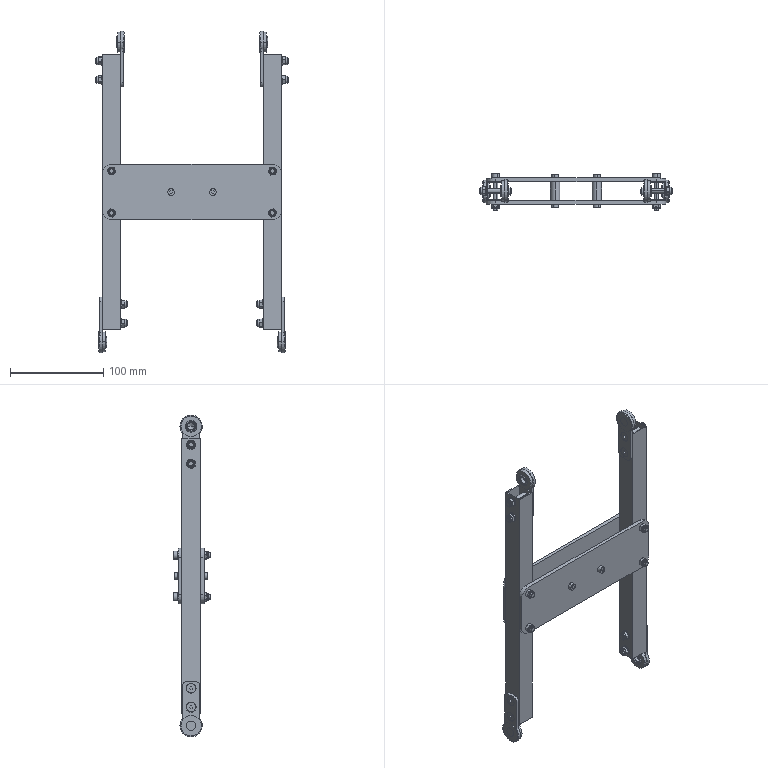Part | SolidWorks | 46 solids | 1092 faces | box 207.8 x 40 x 345.766 mm | volume 168443 mm3 | cylinder 392 | plane 340 | cone 320 | spline 40 | commonest cylinder face diameters 0.4 x84 5 x64 5.3 x48 10 x44 5.2 x32 8 x24